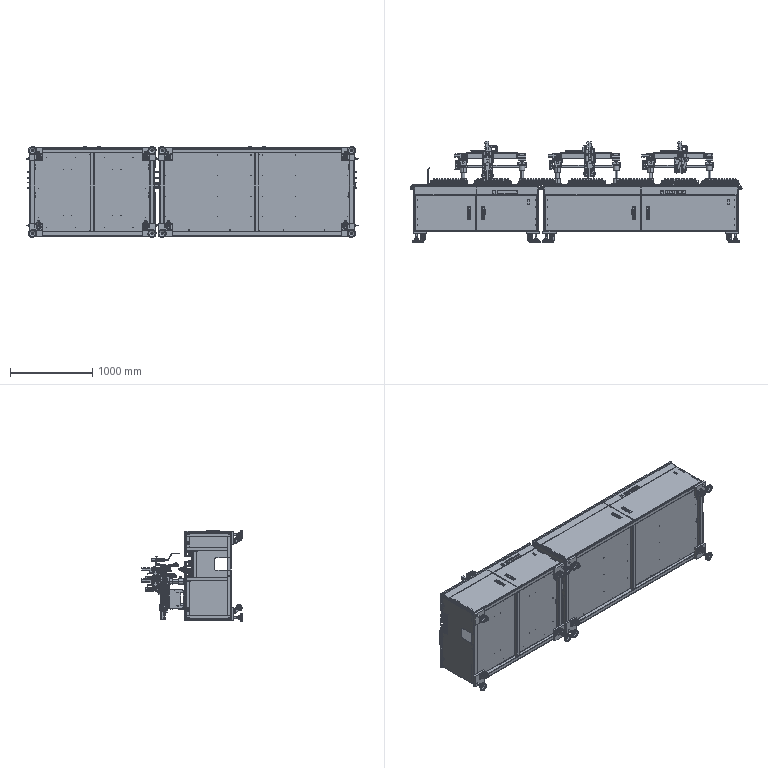Part | NX | features BREP 264 | 1532 solids | 98729 faces | volume 159786594 mm3 | plane 54011 | cylinder 29554 | spline 7768 | cone 5422 | torus 1722 | sphere 252 | commonest cylinder face diameters 0.5 x3472 4 x1688 8 x1606 3 x1526 3.3 x1434 5 x1302